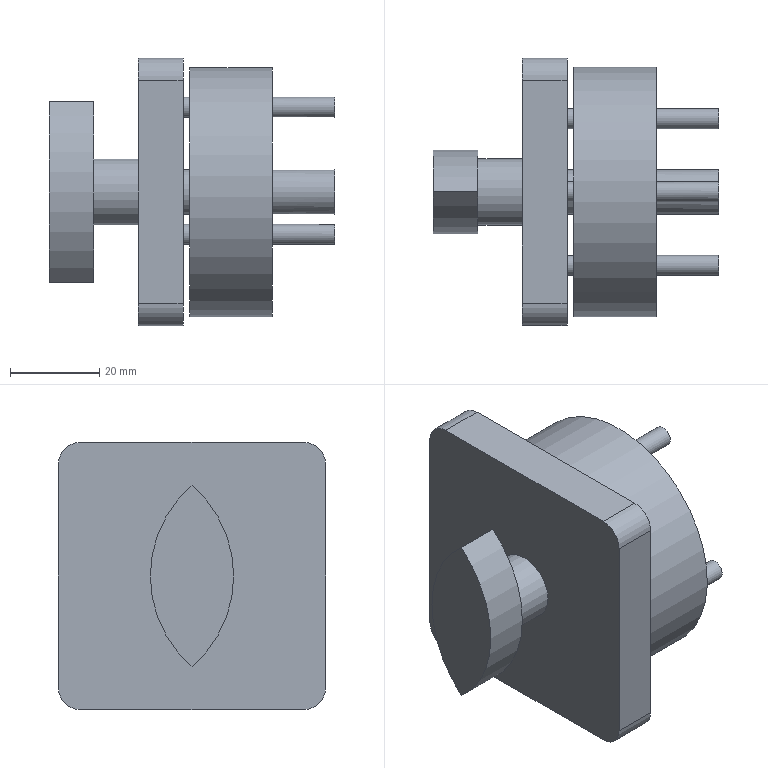Part | STEP file | Power switch | 2 solids | 60 faces | box 64 x 60 x 60 mm | volume 180692 mm3 | cylinder 32 | plane 28 | commonest cylinder face diameters 4.5 x12 10 x12 53.607 x4 15 x2 56 x2